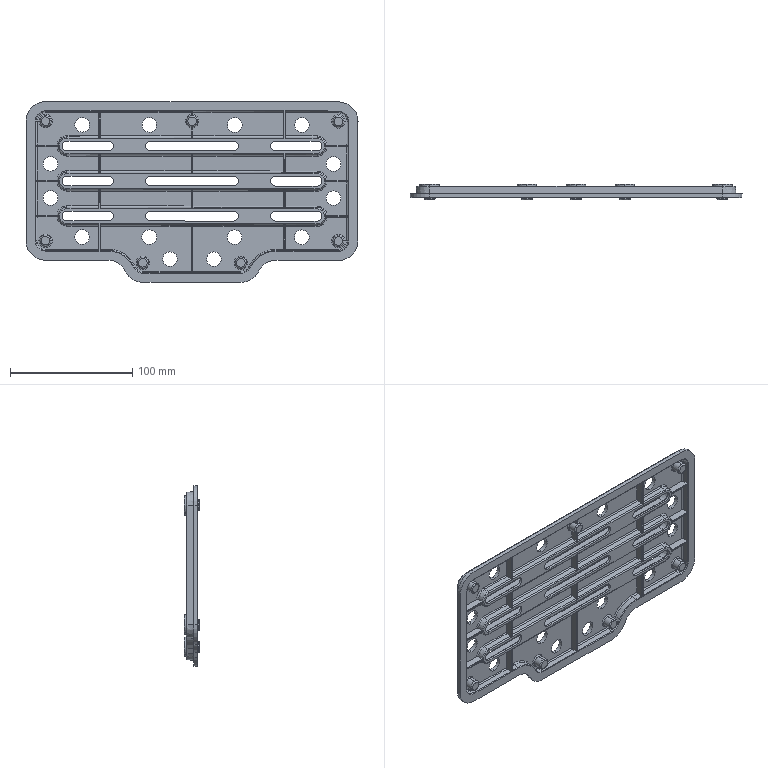Part | SolidWorks | features BaseBody 1 | 1 solid | 641 faces | box 272.077 x 12.8 x 148.126 mm | volume 127916 mm3 | cylinder 317 | plane 198 | torus 97 | cone 27 | spline 2 | commonest cylinder face diameters 2 x74 3.4 x42 12 x42 0.6 x38 7.4 x28 1 x26